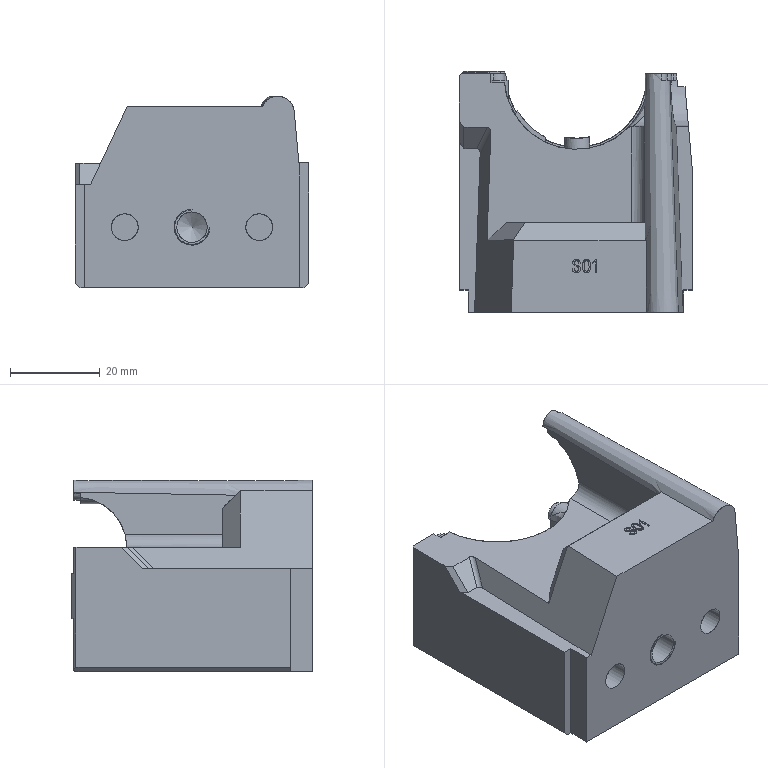NC program | PowerMill | posted with a generic post | part box 52 x 53.756 x 42.711 mm
Lines 1 to 844 of 8909:
%
O0001
N104 ( POWERMILL CB  : 2026004.0)
N105 ( POST VER      : 2026.0.0.5161)
N106 ( OPTION FILE   : FANUC)
N107 ( OUTPUT WORKPLANE : 3)
N108 (  )
N109 ( TOOL LIST )
N110 (-----------------------------------)
N111 ( NO. | ID    | DIA.| TIP RAD|LENGTH)
N112 (-----------------------------------)
N113 (    1|D10_1_1|10.0 |  0.0   |110.76)
N114 (-----------------------------------)
N115 (  )
N116 ( NUMBER OF TOOLPATHS: 1.0 )
N117 ( ESTIMATED PROGRAM DURATION: 0 HOURS 9 MIN 7 SEC)
N118 (  )
N119 G00 G21 G80 G40 G17
N120 G90
N121 G54
N122 G53 Z0.0
N123 (---------------)
N124 ( START TOOLPATH : 17开粗-D10-偏置区域二粗-残留模型 )
N125 (---------------)
N126 ( TOOL NO.    :1 )
N127 ( TOOL TYPE   : ENDMILL)
N128 ( TOOL ID     : D10_1_1)
N129 ( TOOL DIA    : 10.0 LENGTH 110.76)
N130 T1
N131 M6
N132 S3200 M03
N133 G00 G90 X1.5365 Y39.0066
N134 G43 Z63.71 H1
N135
N136 G05 P10000 R8
N137 Z46.5605
N138 G01 Z43.5605 F2400.0
N139 X1.5191 Y38.9966 F4000.0
N140 G03 X0.0179 Y36.3993 I1.4988 J-2.5988
N141 G01 X0.0152 Y30.5762
N142 X0.0124 Y24.6701
N143 X0.0097 Y18.7983
N144 X-12.5642 Y18.8042
N145 G03 X-14.5632 Y16.7147 I-0.001 J-2.0
N146 G01 X-14.4663 Y14.5539
N147 G03 X-12.4684 Y12.6434 I1.9979 J0.0895
N148 G01 X12.4878 Y12.6427
N149 G03 X14.4859 Y14.5546 I0.0 J2.0
N150 G01 X14.5806 Y16.7043
N151 G03 X12.5835 Y18.7924 I-1.998 J0.0881
N152 G01 X0.0097 Y18.7983
N153 X0.0124 Y24.6701
N154 X-18.5964 Y24.6782
N155 G03 X-20.5966 Y22.6242 I-0.0009 J-2.0
N156 G01 X-20.3135 Y12.1442
N157 G03 X-20.0644 Y10.2278 I9.4623 J0.2557
N158 G01 X-19.6039 Y8.2748
N159 G03 X-17.6573 Y6.7338 I1.9466 J0.459
N160 G01 X17.6509 Y6.7331
N161 G03 X19.5844 Y8.2214 I0.0001 J2.0
N162 G01 X20.0778 Y10.0859
N163 G03 X20.3243 Y11.8013 I-7.2377 J1.9153
N164 G01 X20.6129 Y22.6086
N165 G03 X18.6145 Y24.662 I-1.9993 J0.0534
N166 G01 X0.0124 Y24.6701
N167 X0.0152 Y30.5762
N168 X-24.3713 Y30.587
N169 G03 X-26.3717 Y28.632 I-0.0009 J-2.0
N170 G01 X-26.7403 Y12.2427
N171 G03 X-25.4556 Y6.1389 I13.6806 J-0.3076
N172 G01 X-23.3909 Y1.7233
N173 G03 X-21.5792 Y0.5705 I1.8117 J0.8472
N174 G01 X21.5809 Y0.5709
N175 G03 X23.3943 Y1.7274 I0.0 J2.0
N176 G01 X25.6643 Y6.6076
N177 G03 X26.7506 Y11.7759 I-10.5826 J4.9225
N178 G01 X26.396 Y28.6074
N179 G03 X24.3973 Y30.5653 I-1.9995 J-0.0421
N180 G01 X0.0152 Y30.5762
N181 X0.0179 Y36.3993
N182 G03 X-1.4809 Y38.998 I-3.0 J0.0014
N183 G01 X1.7278 Y38.9978 Z43.4109
N184 X1.7104 Y38.9879
N185 G03 X0.1928 Y36.4001 I1.4824 J-2.6082
N186 G01 X0.1523 Y30.4254
N187 X0.1124 Y24.554
N188 X0.0728 Y18.7124
N189 X-12.1305 Y18.7952
N190 G03 X-14.1325 Y16.58 I-0.0136 J-1.9999
N191 G01 X-13.8901 Y14.3413
N192 G03 X-11.8999 Y12.5565 I1.9883 J0.2152
N193 G01 X12.0201 Y12.5791
N194 G03 X14.0041 Y14.3424 I-0.0019 J2.0
N195 G01 X14.2485 Y16.393
N196 G03 X12.2761 Y18.6296 I-1.986 J0.2366
N197 G01 X0.0728 Y18.7124
N198 X0.1124 Y24.554
N199 X-18.3661 Y24.6758
N200 G03 X-20.375 Y22.5457 I-0.0132 J-2.0
N201 G01 X-19.5534 Y9.9449
N202 X-19.5127 Y9.6532
N203 X-19.1981 Y8.1954
N204 G03 X-17.2417 Y6.6172 I1.955 J0.4218
N205 G01 X17.5494 Y6.642
N206 G03 X19.5429 Y8.4988 I-0.0014 J2.0
N207 G01 X20.5334 Y22.2893
N208 G03 X18.5517 Y24.4325 I-1.9948 J0.1432
N209 G01 X0.1124 Y24.554
N210 X0.1523 Y30.4254
N211 X-24.3589 Y30.5872
N212 G03 X-26.3717 Y28.5467 I-0.0132 J-1.9999
N213 G01 X-25.9679 Y8.6375
N214 G03 X-25.8035 Y7.8829 I1.9996 J0.0405
N215 G01 X-23.1199 Y1.6893
N216 G03 X-21.247 Y0.4623 I1.8688 J0.8097
N217 G01 X21.2498 Y0.5492
N218 G03 X22.2801 Y0.8374 I-0.0041 J2.0
N219 G01 X23.1534 Y1.3651
N220 G03 X24.0158 Y2.4425 I-1.0343 J1.7118
N221 G01 X25.8348 Y7.8805
N222 G03 X25.937 Y8.4468 I-1.8967 J0.6345
N223 G01 X26.6112 Y28.1956
N224 G03 X24.6255 Y30.2638 I-1.9989 J0.0682
N225 G01 X0.1523 Y30.4254
N226 X0.1928 Y36.4001
N227 G03 X-1.2895 Y39.0083 I-2.9999 J0.0203
N228 G01 X1.7437 Y38.9973 Z43.2614
N229 X1.7263 Y38.9874
N230 G03 X0.2074 Y36.4003 I1.481 J-2.6089
N231 G01 X0.1639 Y30.4132
N232 X0.1212 Y24.5423
N233 X0.0788 Y18.7012
N234 X-12.1298 Y18.79
N235 G03 X-14.1326 Y16.5742 I-0.0145 J-2.0
N236 G01 X-13.8902 Y14.3407
N237 G03 X-11.8999 Y12.5566 I1.9883 J0.2159
N238 G01 X12.0271 Y12.5801
N239 G03 X14.0105 Y14.3382 I-0.002 J2.0
N240 G01 X14.2581 Y16.3706
N241 G03 X12.2873 Y18.6125 I-1.9853 J0.2419
N242 G01 X0.0788 Y18.7012
N243 X0.1212 Y24.5423
N244 X-18.3653 Y24.6733
N245 G03 X-20.3753 Y22.5431 I-0.0142 J-2.0
N246 G01 X-19.5534 Y9.9449
N247 X-19.5126 Y9.6532
N248 X-19.198 Y8.1953
N249 G03 X-17.2416 Y6.6172 I1.955 J0.4219
N250 G01 X17.5494 Y6.6421
N251 G03 X19.5426 Y8.496 I-0.0015 J2.0
N252 G01 X20.5515 Y22.2655
N253 G03 X18.571 Y24.4116 I-1.9947 J0.1461
N254 G01 X0.1212 Y24.5423
N255 X0.1639 Y30.4132
N256 X-24.3578 Y30.5874
N257 G03 X-26.3716 Y28.5469 I-0.0142 J-2.0
N258 G01 X-25.9679 Y8.6375
N259 G03 X-25.8035 Y7.8829 I1.9995 J0.0405
N260 G01 X-23.1199 Y1.6895
N261 G03 X-21.2465 Y0.4622 I1.8692 J0.8099
N262 G01 X21.2498 Y0.5493
N263 G03 X22.2801 Y0.8375 I-0.0041 J2.0
N264 G01 X23.1533 Y1.3652
N265 G03 X24.0155 Y2.4424 I-1.0344 J1.7117
N266 G01 X25.8348 Y7.8805
N267 G03 X25.9369 Y8.4441 I-1.8966 J0.6345
N268 G01 X26.6367 Y28.1683
N269 G03 X24.6522 Y30.2392 I-1.9987 J0.071
N270 G01 X0.1639 Y30.4132
N271 X0.2074 Y36.4003
N272 G03 X-1.2736 Y39.0092 I-2.9999 J0.0218
N273 G01 X1.7432 Y38.9975 Z43.1119
N274 X1.7258 Y38.9876
N275 G03 X0.207 Y36.4005 I1.4811 J-2.6089
N276 G01 X0.1636 Y30.4136
N277 X0.121 Y24.5427
N278 X0.0786 Y18.7016
N279 X-12.1298 Y18.7902
N280 G03 X-14.1326 Y16.5744 I-0.0145 J-1.9999
N281 G01 X-13.8902 Y14.3407
N282 G03 X-11.8999 Y12.5565 I1.9884 J0.2158
N283 G01 X12.0268 Y12.5802
N284 G03 X14.0102 Y14.3384 I-0.0019 J2.0
N285 G01 X14.2578 Y16.3713
N286 G03 X12.287 Y18.613 I-1.9854 J0.2418
N287 G01 X0.0786 Y18.7016
N288 X0.121 Y24.5427
N289 X-18.3653 Y24.6734
N290 G03 X-20.3752 Y22.5433 I-0.0141 J-1.9999
N291 G01 X-19.5534 Y9.945
N292 X-19.5126 Y9.6532
N293 X-19.1979 Y8.1952
N294 G03 X-17.2415 Y6.6172 I1.955 J0.422
N295 G01 X17.5493 Y6.6422
N296 G03 X19.5425 Y8.4961 I-0.0014 J2.0
N297 G01 X20.5509 Y22.2662
N298 G03 X18.5704 Y24.4122 I-1.9946 J0.1461
N299 G01 X0.121 Y24.5427
N300 X0.1636 Y30.4136
N301 X-24.3578 Y30.5875
N302 G03 X-26.3715 Y28.547 I-0.0141 J-2.0
N303 G01 X-25.9679 Y8.6376
N304 G03 X-25.8034 Y7.8829 I1.9996 J0.0405
N305 G01 X-23.1199 Y1.6897
N306 G03 X-21.246 Y0.4622 I1.8697 J0.8102
N307 G01 X21.2498 Y0.5493
N308 G03 X22.2801 Y0.8376 I-0.0041 J2.0
N309 G01 X23.1531 Y1.3652
N310 G03 X24.0153 Y2.4423 I-1.0345 J1.7117
N311 G01 X25.8348 Y7.8804
N312 G03 X25.9369 Y8.4442 I-1.8966 J0.6346
N313 G01 X26.6359 Y28.1692
N314 G03 X24.6513 Y30.2399 I-1.9987 J0.0708
N315 G01 X0.1636 Y30.4136
N316 X0.207 Y36.4005
N317 G03 X-1.2741 Y39.0094 I-2.9999 J0.0217
N318 G01 X1.7531 Y38.997 Z42.9623
N319 X1.7357 Y38.9871
N320 G03 X0.2176 Y36.3996 I1.4818 J-2.6085
N321 G01 X0.176 Y30.4423
N322 X0.1349 Y24.5504
N323 X0.0941 Y18.7107
N324 X-12.1304 Y18.7961
N325 G03 X-14.1327 Y16.5807 I-0.014 J-2.0
N326 G01 X-13.8901 Y14.3411
N327 G03 X-11.8996 Y12.5565 I1.9884 J0.2154
N328 G01 X12.0454 Y12.5828
N329 G03 X14.027 Y14.3288 I-0.0022 J2.0
N330 G01 X14.2885 Y16.3715
N331 G03 X12.3187 Y18.6254 I-1.9838 J0.2539
N332 G01 X0.0941 Y18.7107
N333 X0.1349 Y24.5504
N334 X-18.3656 Y24.6784
N335 G03 X-20.3752 Y22.5484 I-0.0138 J-1.9999
N336 G01 X-19.5534 Y9.9451
N337 X-19.5126 Y9.6532
N338 X-19.1978 Y8.1951
N339 G03 X-17.2414 Y6.6171 I1.9549 J0.422
N340 G01 X17.5492 Y6.6423
N341 G03 X19.5419 Y8.4887 I-0.0014 J2.0
N342 G01 X20.6032 Y22.269
N343 G03 X18.6229 Y24.4225 I-1.9941 J0.1536
N344 G01 X0.1349 Y24.5504
N345 X0.176 Y30.4423
N346 X-24.36 Y30.5876
N347 G03 X-26.3715 Y28.5471 I-0.0119 J-2.0
N348 G01 X-25.9679 Y8.6376
N349 G03 X-25.8034 Y7.883 I1.9996 J0.0406
N350 G01 X-23.12 Y1.6902
N351 G03 X-21.2453 Y0.4622 I1.8705 J0.8105
N352 G01 X21.2497 Y0.5494
N353 G03 X22.2801 Y0.8378 I-0.0041 J2.0
N354 G01 X23.1529 Y1.3653
N355 G03 X24.015 Y2.4422 I-1.0345 J1.7116
N356 G01 X25.8348 Y7.8804
N357 G03 X25.9366 Y8.437 I-1.8966 J0.6347
N358 G01 X26.7049 Y28.0971
N359 G03 X24.7561 Y30.1746 I-1.9985 J0.0781
N360 G01 X18.2868 Y30.335
N361 X0.176 Y30.4423
N362 X0.2176 Y36.3996
N363 G03 X-1.2642 Y39.0081 I-2.9999 J0.0209
N364 G00 Z50.8128
N365 G01 X24.7981 Y56.2442 F10000.0
N366 G00 Z45.8128
N367 G01 Z42.8128 F2400.0
N368 X24.7818 Y56.2326 F4000.0
N369 G03 X23.5382 Y53.5025 I1.7426 J-2.442
N370 G01 X23.5458 Y53.4242
N371 X23.5507 Y52.7924
N372 X23.594 Y52.1606
N373 X23.6145 Y51.5288
N374 X23.8877 Y36.997
N375 X24.12 Y24.9925
N376 X24.1645 Y21.8334
N377 X24.1934 Y21.2016
N378 X24.2312 Y18.6743
N379 X24.2648 Y17.4107
N380 X24.3018 Y15.5152
N381 X24.2942 Y14.8834
N382 X24.3263 Y14.2516
N383 X24.5696 Y1.6153
N384 X24.5629 Y0.9834
N385 X24.5639 Y0.9647
N386 X24.5957 Y0.3516
N387 X24.5843 Y-0.2802
N388 X24.5185 Y-0.912
N389 X24.35 Y-1.5438
N390 X24.009 Y-2.3915
N391 X23.7492 Y-2.8075
N392 X23.3772 Y-3.3198
N393 X23.2743 Y-3.4393
N394 X22.7454 Y-3.9427
N395 X22.5827 Y-4.0711
N396 X22.1136 Y-4.391
N397 X21.4992 Y-4.7029
N398 X20.85 Y-4.9286
N399 X20.2181 Y-5.0644
N400 X19.5863 Y-5.133
N401 X18.9545 Y-5.1314
N402 X18.3227 Y-5.1019
N403 X17.6909 Y-4.9883
N404 X17.0591 Y-4.802
N405 X16.8097 Y-4.7029
N406 X16.4272 Y-4.5164
N407 X15.7954 Y-4.1252
N408 X15.1636 Y-3.579
N409 X15.0273 Y-3.4393
N410 X14.5318 Y-2.8
N411 X14.1799 Y-2.1756
N412 X13.9317 Y-1.5438
N413 X13.7748 Y-0.912
N414 X13.7001 Y-0.2802
N415 X13.7058 Y0.9834
N416 X13.6856 Y2.2471
N417 X13.6783 Y2.6491
N418 X7.7919 Y2.5388
N419 G02 X5.7903 Y0.5013 I-1.9996 J-0.0375
N420 G01 X-21.2214 Y0.5283
N421 G02 X-22.2624 Y0.8218 I0.002 J2.0
N422 G01 X-23.1599 Y1.3703
N423 G02 X-24.0144 Y2.445 I1.043 J1.7065
N424 G01 X-25.8465 Y7.9472
N425 G02 X-25.9485 Y8.5368 I1.8976 J0.6318
N426 G01 X-26.3714 Y28.5455
N427 G02 X-24.3657 Y30.5877 I1.9996 J0.0422
N428 G01 X-9.0066 Y30.5405
N429 X-9.0995 Y24.6503
N430 X-9.1922 Y18.7738
N431 X-12.1364 Y18.8202
N432 G03 X-14.1578 Y16.6194 I-0.0315 J-1.9997
N433 G01 X-13.9222 Y14.2872
N434 G03 X-11.9861 Y12.489 I1.9899 J0.2011
N435 G01 X-6.2409 Y12.3343
N436 G03 X-4.1886 Y14.4108 I0.0538 J1.9993
N437 G01 X-4.281 Y16.8048
N438 G03 X-6.248 Y18.7274 I-1.9985 J-0.0772
N439 G01 X-9.1922 Y18.7738
N440 X-9.0995 Y24.6503
N441 X-0.482 Y24.6082
N442 G02 X1.5078 Y22.6498 I-0.0097 J-2.0
N443 G01 X1.8037 Y8.4257
N444 G02 X-0.2235 Y6.3843 I-1.9995 J-0.0416
N445 G01 X-17.5632 Y6.6238
N446 G02 X-19.532 Y8.5049 I0.0276 J1.9998
N447 G01 X-20.3688 Y22.5769
N448 G02 X-18.3626 Y24.6956 I1.9965 J0.1187
N449 G01 X-9.0995 Y24.6503
N450 X-9.0066 Y30.5405
N451 X5.3112 Y30.4965
N452 G02 X7.3047 Y28.534 I-0.0061 J-2.0
N453 G01 X7.7919 Y2.5388
N454 X13.6783 Y2.6491
N455 X13.1981 Y29.4152
N456 X12.9886 Y40.7879
N457 X12.779 Y51.5288
N458 X12.7688 Y53.4242
N459 X12.7944 Y53.7176
N460 G03 X11.5259 Y56.4362 I-2.9887 J0.2608
N461 G00 Z50.6633
N462 G01 X25.8509 Y46.8237 F10000.0
N463 G00 Z45.6633
N464 G01 Z42.6633 F2400.0
N465 X25.8338 Y46.8133 F4000.0
N466 G03 X24.388 Y44.1847 I1.5536 J-2.5663
N467 G01 X25.311 Y-0.2802
N468 X25.237 Y-0.912
N469 X25.0806 Y-1.5438
N470 X24.8336 Y-2.1756
N471 X24.4809 Y-2.8075
N472 X23.9931 Y-3.4393
N473 X23.3772 Y-4.0169
N474 X22.7454 Y-4.4492
N475 X22.2507 Y-4.7029
N476 X21.4818 Y-4.9806
N477 X20.85 Y-5.1193
N478 X20.2181 Y-5.1887
N479 X19.5863 Y-5.2063
N480 X18.3227 Y-5.2032
N481 X17.6909 Y-5.1561
N482 X17.0591 Y-5.046
N483 X16.4272 Y-4.8633
N484 X16.0237 Y-4.7029
N485 X15.7954 Y-4.5939
N486 X15.1636 Y-4.2183
N487 X14.9591 Y-4.0711
N488 X14.5318 Y-3.7025
N489 X14.2718 Y-3.4393
N490 X13.9 Y-2.977
N491 X13.7826 Y-2.8075
N492 X13.4293 Y-2.1756
N493 X13.1821 Y-1.5438
N494 X13.0248 Y-0.912
N495 X12.9511 Y-0.2802
N496 X12.9106 Y2.6316
N497 X7.0274 Y2.5364
N498 G02 X4.9833 Y0.5045 I-1.9997 J-0.0324
N499 G01 X-20.4191 Y1.0678
N500 X-20.7511 Y1.103
N501 X-21.9838 Y1.4406
N502 G02 X-23.2515 Y2.5082 I0.5388 J1.926
N503 G01 X-25.7742 Y7.8171
N504 G02 X-25.9673 Y8.6349 I1.8065 J0.8584
N505 G01 X-26.3713 Y28.5473
N506 G02 X-24.3653 Y30.5878 I1.9995 J0.0406
N507 G01 X-9.3219 Y30.5392
N508 X-9.4283 Y24.6495
N509 X-9.5344 Y18.7757
N510 X-12.1053 Y18.8221
N511 G03 X-14.1247 Y16.5643 I-0.0361 J-1.9996
N512 G01 X-13.8775 Y14.665
N513 G03 X-12.0232 Y12.9273 I1.9833 J0.2581
N514 G01 X-7.0277 Y12.6045
N515 G03 X-4.901 Y14.6949 I0.129 J1.9958
N516 G01 X-5.0017 Y16.8241
N517 G03 X-6.9634 Y18.7293 I-1.9978 J-0.0945
N518 G01 X-9.5344 Y18.7757
N519 X-9.4283 Y24.6495
N520 X-1.1929 Y24.6084
N521 G02 X0.7967 Y22.6465 I-0.01 J-2.0
N522 G01 X1.066 Y8.5393
N523 G02 X-1.0163 Y6.5029 I-1.9997 J-0.0381
N524 G01 X-17.4499 Y7.1821
N525 G02 X-19.3293 Y8.7925 I0.0826 J1.9983
N526 G01 X-19.5496 Y9.9282
N527 X-20.3726 Y22.565
N528 G02 X-18.3668 Y24.6943 I1.9958 J0.1293
N529 G01 X-9.4283 Y24.6495
N530 X-9.3219 Y30.5392
N531 X4.6135 Y30.494
N532 G02 X6.6068 Y28.5264 I-0.0064 J-2.0
N533 G01 X7.0274 Y2.5364
N534 X12.9106 Y2.6316
N535 X12.9071 Y2.8789
N536 X12.3349 Y39.5243
N537 X12.1563 Y51.5288
N538 X12.1654 Y52.1606
N539 X12.1399 Y53.4242
N540 X12.1427 Y53.4555
N541 G03 X10.8844 Y56.1788 I-2.9876 J0.272
N542 G00 Z50.5137
N543 G01 X26.3161 Y42.059 F10000.0
N544 G00 Z45.5137
N545 G01 Z42.5137 F2400.0
N546 X26.299 Y42.0486 F4000.0
N547 G03 X24.8565 Y39.4182 I1.5567 J-2.5644
N548 G01 X25.7153 Y0.3516
N549 X25.717 Y-0.2802
N550 X25.6435 Y-0.912
N551 X25.4875 Y-1.5438
N552 X25.2727 Y-2.1031
N553 X24.8912 Y-2.8075
N554 X24.6409 Y-3.1542
N555 X24.4065 Y-3.4393
N556 X24.009 Y-3.8349
N557 X23.7278 Y-4.0711
N558 X23.3772 Y-4.3209
N559 X22.6869 Y-4.7029
N560 X22.1136 Y-4.9269
N561 X21.4818 Y-5.0921
N562 X20.85 Y-5.1809
N563 X20.2181 Y-5.2059
N564 X19.6527 Y-5.2044
N565 X19.5863 Y-5.2063
N566 X18.3227 Y-5.2031
N567 X18.2939 Y-5.201
N568 X17.6909 Y-5.1994
N569 X17.0591 Y-5.1379
N570 X16.4272 Y-5.004
N571 X15.7954 Y-4.7899
N572 X15.593 Y-4.7029
N573 X15.1636 Y-4.4822
N574 X14.5461 Y-4.0711
N575 X13.9 Y-3.4764
N576 X13.377 Y-2.8075
N577 X13.0242 Y-2.1756
N578 X12.7779 Y-1.5438
N579 X12.6363 Y-0.9846
N580 X12.5478 Y-0.2802
N581 X12.5064 Y2.6233
N582 X6.6265 Y2.5351
N583 G02 X4.5816 Y0.5056 I-1.9998 J-0.03
N584 G01 X-20.3244 Y1.0678
N585 X-20.5926 Y1.092
N586 X-20.855 Y1.1519
N587 X-22.015 Y1.5006
N588 G02 X-23.2415 Y2.5489 I0.5757 J1.9153
N589 G01 X-25.7686 Y7.8018
N590 G02 X-25.9659 Y8.6282 I1.8022 J0.8671
N591 G01 X-26.3713 Y28.5472
N592 G02 X-24.3655 Y30.5879 I1.9996 J0.0407
N593 G01 X-9.5033 Y30.5416
N594 X-9.6138 Y24.6525
N595 X-9.7239 Y18.7791
N596 X-12.1031 Y18.8237
N597 G03 X-14.1238 Y16.5652 I-0.0375 J-1.9997
N598 G01 X-13.8756 Y14.6636
N599 G03 X-12.0276 Y12.927 I1.9832 J0.2588
N600 G01 X-7.4206 Y12.615
N601 G03 X-5.2876 Y14.7014 I0.1351 J1.9954
N602 G01 X-5.3844 Y16.8258
N603 G03 X-7.3448 Y18.7344 I-1.9979 J-0.091
N604 G01 X-9.7239 Y18.7791
N605 X-9.6138 Y24.6525
N606 X-1.5696 Y24.6133
N607 G02 X0.4203 Y22.649 I-0.0097 J-2.0
N608 G01 X0.6716 Y8.5407
N609 G02 X-1.4127 Y6.5068 I-1.9997 J-0.0357
N610 G01 X-17.4396 Y7.1857
N611 G02 X-19.3128 Y8.7752 I0.0846 J1.9982
N612 G01 X-19.5482 Y9.9273
N613 X-20.3722 Y22.5657
N614 G02 X-18.3667 Y24.695 I1.9958 J0.1294
N615 G01 X-9.6138 Y24.6525
N616 X-9.5033 Y30.5416
N617 X4.2428 Y30.4988
N618 G02 X6.2363 Y28.5288 I-0.0063 J-2.0
N619 G01 X6.6265 Y2.5351
N620 X12.5064 Y2.6233
N621 X11.8762 Y46.9023
N622 G03 X10.3394 Y49.4788 I-2.9997 J-0.0427
N623 G00 Z50.3642
N624 G01 X26.6593 Y38.9687 F10000.0
N625 G00 Z45.3642
N626 G01 Z42.3642 F2400.0
N627 X26.6422 Y38.9583 F4000.0
N628 G03 X25.2029 Y36.3261 I1.5599 J-2.5626
N629 G01 X25.7744 Y11.7243
N630 X26.0158 Y0.9834
N631 X26.0338 Y-0.2802
N632 X25.9599 Y-0.912
N633 X25.8048 Y-1.5438
N634 X25.5579 Y-2.1756
N635 X25.2085 Y-2.8075
N636 X24.7245 Y-3.4393
N637 X24.0456 Y-4.0711
N638 X23.3772 Y-4.5133
N639 X23.0026 Y-4.7029
N640 X22.7454 Y-4.8121
N641 X22.1136 Y-5.0207
N642 X21.4818 Y-5.148
N643 X20.85 Y-5.2023
N644 X20.2961 Y-5.2027
N645 X20.2181 Y-5.2058
N646 X19.6527 Y-5.2044
N647 X19.5863 Y-5.2062
N648 X18.6982 Y-5.204
N649 X17.6909 Y-5.2048
N650 X17.0591 Y-5.1807
N651 X16.4272 Y-5.0868
N652 X15.7954 Y-4.9166
N653 X15.2597 Y-4.7029
N654 X14.5318 Y-4.2933
N655 X14.2252 Y-4.0711
N656 X13.9 Y-3.7945
N657 X13.5504 Y-3.4393
N658 X13.2682 Y-3.0932
N659 X13.0675 Y-2.8075
N660 X12.7171 Y-2.1756
N661 X12.4716 Y-1.5438
N662 X12.3174 Y-0.912
N663 X12.2428 Y-0.2802
N664 X12.2042 Y2.6156
N665 X6.3237 Y2.5337
N666 G02 X4.2783 Y0.5063 I-1.9998 J-0.0279
N667 G01 X-20.3249 Y1.0678
N668 X-20.5928 Y1.092
N669 X-20.855 Y1.1519
N670 X-22.015 Y1.5006
N671 G02 X-23.2415 Y2.5489 I0.5757 J1.9153
N672 G01 X-25.7686 Y7.8018
N673 G02 X-25.9659 Y8.6282 I1.8023 J0.8671
N674 G01 X-26.3712 Y28.5474
N675 G02 X-24.3654 Y30.588 I1.9995 J0.0406
N676 G01 X-9.6369 Y30.542
N677 X-9.7514 Y24.6532
N678 X-9.8657 Y18.7803
N679 X-12.1017 Y18.8238
N680 G03 X-14.1237 Y16.5652 I-0.0389 J-1.9997
N681 G01 X-13.8749 Y14.6601
N682 G03 X-12.0315 Y12.924 I1.9831 J0.259
N683 G01 X-7.7153 Y12.6218
N684 G03 X-5.5776 Y14.7045 I0.1397 J1.9951
N685 G01 X-5.6706 Y16.8248
N686 G03 X-7.6298 Y18.7368 I-1.9981 J-0.0877
N687 G01 X-9.8657 Y18.7803
N688 X-9.7514 Y24.6532
N689 X-1.8501 Y24.6149
N690 G02 X0.14 Y22.6482 I-0.0097 J-2.0
N691 G01 X0.3748 Y8.541
N692 G02 X-1.7108 Y6.5096 I-1.9998 J-0.0333
N693 G01 X-17.4404 Y7.1851
N694 G02 X-19.3123 Y8.7741 I0.0858 J1.9982
N695 G01 X-19.5481 Y9.927
N696 X-20.3722 Y22.5658
N697 G02 X-18.3666 Y24.6951 I1.9958 J0.1293
N698 G01 X-9.7514 Y24.6532
N699 X-9.6369 Y30.542
N700 X3.9678 Y30.4995
N701 G02 X5.9614 Y28.5274 I-0.0062 J-2.0
N702 G01 X6.3237 Y2.5337
N703 X12.2042 Y2.6156
N704 X11.8813 Y26.8879
N705 X11.5887 Y49.2077
N706 G03 X10.0547 Y51.7858 I-2.9998 J-0.0394
N707 G00 Z50.2147
N708 G01 X26.8772 Y39.0077 F10000.0
N709 G00 Z45.2147
N710 G01 Z42.2147 F2400.0
N711 X26.8601 Y38.9973 F4000.0
N712 G03 X25.4217 Y36.3646 I1.5608 J-2.562
N713 G01 X26.2554 Y0.9834
N714 X26.2798 Y-0.2802
N715 X26.2049 Y-0.912
N716 X26.049 Y-1.5438
N717 X25.804 Y-2.1756
N718 X25.4536 Y-2.8075
N719 X25.2727 Y-3.0669
N720 X24.9704 Y-3.4393
N721 X24.6409 Y-3.7749
N722 X24.2933 Y-4.0711
N723 X24.009 Y-4.2793
N724 X23.2612 Y-4.7029
N725 X22.7454 Y-4.9105
N726 X22.1136 Y-5.0854
N727 X21.4818 Y-5.1814
N728 X20.85 Y-5.205
N729 X20.2619 Y-5.2041
N730 X20.2181 Y-5.2058
N731 X19.6527 Y-5.2043
N732 X19.5863 Y-5.2062
N733 X18.6982 Y-5.204
N734 X17.6909 Y-5.2048
N735 X17.5541 Y-5.1995
N736 X17.0591 Y-5.1987
N737 X16.4272 Y-5.1343
N738 X15.7954 Y-4.995
N739 X15.1636 Y-4.774
N740 X14.5318 Y-4.4553
N741 X13.9665 Y-4.0711
N742 X13.2682 Y-3.4134
N743 X12.8096 Y-2.8075
N744 X12.6363 Y-2.5214
N745 X12.4602 Y-2.1756
N746 X12.215 Y-1.5438
N747 X12.0582 Y-0.912
N748 X11.985 Y-0.2802
N749 X11.948 Y2.6102
N750 X6.0673 Y2.5327
N751 G02 X4.0214 Y0.5069 I-1.9999 J-0.0264
N752 G01 X-20.3253 Y1.0678
N753 X-20.593 Y1.092
N754 X-20.855 Y1.1519
N755 X-22.015 Y1.5006
N756 G02 X-23.2415 Y2.5489 I0.5757 J1.9153
N757 G01 X-25.7686 Y7.8018
N758 G02 X-25.9659 Y8.6282 I1.8022 J0.8671
N759 G01 X-26.3712 Y28.5475
N760 G02 X-24.3653 Y30.5881 I1.9996 J0.0406
N761 G01 X-9.7494 Y30.5423
N762 X-9.8682 Y24.6538
N763 X-9.9867 Y18.7811
N764 X-12.1002 Y18.8238
N765 G03 X-14.1237 Y16.565 I-0.0403 J-1.9996
N766 G01 X-13.8744 Y14.657
N767 G03 X-12.0353 Y12.9214 I1.9832 J0.2592
N768 G01 X-7.9671 Y12.6275
N769 G03 X-5.8248 Y14.7077 I0.1441 J1.9948
N770 G01 X-5.9153 Y16.8243
N771 G03 X-7.8731 Y18.7385 I-1.9981 J-0.0854
N772 G01 X-9.9867 Y18.7811
N773 X-9.8682 Y24.6538
N774 X-2.0906 Y24.616
N775 G02 X-0.1006 Y22.6477 I-0.0097 J-2.0
N776 G01 X0.1225 Y8.5415
N777 G02 X-1.9641 Y6.5118 I-1.9997 J-0.0316
N778 G01 X-17.4411 Y7.1847
N779 G02 X-19.3118 Y8.7731 I0.0869 J1.9981
N780 G01 X-19.5481 Y9.9267
N781 X-20.3721 Y22.5658
N782 G02 X-18.3666 Y24.6951 I1.9958 J0.1294
N783 G01 X-9.8682 Y24.6538
N784 X-9.7494 Y30.5423
N785 X3.7312 Y30.5001
N786 G02 X5.7248 Y28.5264 I-0.0062 J-2.0
N787 G01 X6.0673 Y2.5327
N788 X11.948 Y2.6102
N789 X11.6943 Y22.4652
N790 X11.4455 Y43.7194
N791 G03 X9.9152 Y46.2998 I-2.9998 J-0.0351
N792 G00 Z50.0652
N793 G01 X27.0522 Y39.0235 F10000.0
N794 G00 Z45.0652
N795 G01 Z42.0652 F2400.0
N796 X27.0352 Y39.0131 F4000.0
N797 G03 X25.6002 Y36.3785 I1.5641 J-2.56
N798 G01 X26.4961 Y0.3516
N799 X26.4958 Y-0.2802
N800 X26.4233 Y-0.912
N801 X26.2681 Y-1.5438
N802 X26.0225 Y-2.1756
N803 X25.9045 Y-2.4158
N804 X25.6738 Y-2.8075
N805 X25.2727 Y-3.3465
N806 X24.6409 Y-3.9728
N807 X24.009 Y-4.4243
N808 X23.4875 Y-4.7029
N809 X22.7454 Y-4.9826
N810 X22.1136 Y-5.1281
N811 X21.4818 Y-5.197
N812 X21.0454 Y-5.1977
N813 X20.85 Y-5.205
N814 X20.2618 Y-5.204
N815 X20.2181 Y-5.2057
N816 X19.6527 Y-5.2043
N817 X19.5863 Y-5.2061
N818 X18.6982 Y-5.2039
N819 X17.6909 Y-5.2047
N820 X17.6336 Y-5.2025
N821 X17.0591 Y-5.2033
N822 X16.4272 Y-5.1678
N823 X15.7954 Y-5.0563
N824 X15.1636 Y-4.8632
N825 X14.7805 Y-4.7029
N826 X14.5318 Y-4.5788
N827 X13.9 Y-4.183
N828 X13.7526 Y-4.0711
N829 X13.2682 Y-3.6385
N830 X13.0809 Y-3.4393
N831 X12.6363 Y-2.8646
N832 X12.2506 Y-2.1756
N833 X12.0045 Y-1.5365
N834 X11.849 Y-0.912
N835 X11.7766 Y-0.2802
N836 X11.7663 Y0.3516
N837 X11.7399 Y2.604
N838 X5.8609 Y2.5315
N839 G02 X3.8147 Y0.5074 I-1.9998 J-0.0246
N840 G01 X-20.3257 Y1.0678
N841 X-20.5931 Y1.092
N842 X-20.855 Y1.1519
N843 X-22.015 Y1.5006
N844 G02 X-23.2415 Y2.5489 I0.5757 J1.9153
N845 G01 X-25.7686 Y7.8018
N846 G02 X-25.9659 Y8.6282 I1.8022 J0.8671
N847 G01 X-26.3711 Y28.5476
N848 G02 X-24.3653 Y30.5882 I1.9996 J0.0407
N849 G01 X-9.8384 Y30.5427
N850 X-9.9604 Y24.6545
N851 X-10.0821 Y18.7821
N852 X-12.0991 Y18.8239
N853 G03 X-14.1236 Y16.5651 I-0.0414 J-1.9996
N854 G01 X-13.8739 Y14.6546
N855 G03 X-12.0385 Y12.9194 I1.9831 J0.2593
N856 G01 X-8.167 Y12.6325
N857 G03 X-6.021 Y14.7096 I0.1477 J1.9946
N858 G01 X-6.1083 Y16.8233
N859 G03 X-8.0652 Y18.7403 I-1.9983 J-0.0826
N860 G01 X-10.0821 Y18.7821
N861 X-9.9604 Y24.6545
N862 X-2.279 Y24.6173
N863 G02 X-0.289 Y22.647 I-0.0097 J-2.0
N864 G01 X-0.0791 Y8.5417
N865 G02 X-2.1666 Y6.5138 I-1.9998 J-0.0298
N866 G01 X-17.4416 Y7.1843
N867 G02 X-19.3114 Y8.7723 I0.0877 J1.9981
N868 G01 X-19.5481 Y9.9265
N869 X-20.3721 Y22.5659
N870 G02 X-18.3666 Y24.6952 I1.9958 J0.1294
N871 G01 X-9.9604 Y24.6545
N872 X-9.8384 Y30.5427
N873 X3.5472 Y30.5007
N874 G02 X5.5408 Y28.5253 I-0.0063 J-2.0
N875 G01 X5.8609 Y2.5315
N876 X11.7399 Y2.604
N877 X11.3444 Y36.3652
N878 X11.2732 Y42.8253
N879 G03 X9.7447 Y45.4067 I-2.9998 J-0.0331
N880 G00 Z49.9156
N881 G01 X17.6127 Y-7.1429 F10000.0
N882 G00 Z44.9156
N883 G01 Z41.9156 F2400.0
N884 X17.6074 Y-7.1236 F4000.0
N885 G03 X15.476 Y-5.0124 I-2.894 J-0.7903
N886 G01 X15.1636 Y-4.9303
N887 X14.5877 Y-4.7029
N888 X13.9 Y-4.3167
N889 X13.5598 Y-4.0711
N890 X13.2682 Y-3.8232
N891 X12.8892 Y-3.4393
N892 X12.6363 Y-3.1327
N893 X12.4071 Y-2.8075
N894 X12.0591 Y-2.1756
N895 X11.8146 Y-1.5438
N896 X11.6596 Y-0.912
N897 X11.5857 Y-0.2802
N898 X11.5522 Y2.5996
N899 X5.6708 Y2.5308
N900 G02 X3.6242 Y0.5079 I-1.9999 J-0.0235
N901 G01 X-20.326 Y1.0678
N902 X-20.5933 Y1.0921
N903 X-20.855 Y1.1519
N904 X-22.015 Y1.5006
N905 G02 X-23.2415 Y2.5489 I0.5757 J1.9153
N906 G01 X-25.7686 Y7.8018
N907 G02 X-25.9659 Y8.6282 I1.8023 J0.8671
N908 G01 X-26.3711 Y28.5477
N909 G02 X-24.3652 Y30.5883 I1.9996 J0.0407
N910 G01 X-9.9202 Y30.5429
N911 X-10.0459 Y24.655
N912 X-10.1713 Y18.7828
N913 X-12.0978 Y18.8239
N914 G03 X-14.1236 Y16.565 I-0.0427 J-1.9995
N915 G01 X-13.8734 Y14.6523
N916 G03 X-12.0419 Y12.9174 I1.9831 J0.2594
N917 G01 X-8.3538 Y12.637
N918 G03 X-6.2038 Y14.712 I0.1516 J1.9943
N919 G01 X-6.2891 Y16.8229
N920 G03 X-8.2447 Y18.7417 I-1.9983 J-0.0808
N921 G01 X-10.1713 Y18.7828
N922 X-10.0459 Y24.655
N923 X-2.4565 Y24.6182
N924 G02 X-0.4664 Y22.6466 I-0.0097 J-2.0
N925 G01 X-0.2659 Y8.542
N926 G02 X-2.3542 Y6.5156 I-1.9998 J-0.0284
N927 G01 X-17.4421 Y7.184
N928 G02 X-19.3111 Y8.7716 I0.0885 J1.998
N929 G01 X-19.548 Y9.9263
N930 X-20.3721 Y22.566
N931 G02 X-18.3666 Y24.6953 I1.9958 J0.1293
N932 G01 X-10.0459 Y24.655
N933 X-9.9202 Y30.5429
N934 X3.3729 Y30.5011
N935 G02 X5.3665 Y28.5246 I-0.0063 J-2.0
N936 G01 X5.6708 Y2.5308
N937 X11.5522 Y2.5996
N938 X11.3654 Y18.6743
N939 X11.1153 Y42.9555
N940 G03 X9.5886 Y45.538 I-2.9998 J-0.0309
N941 G00 Z49.7661